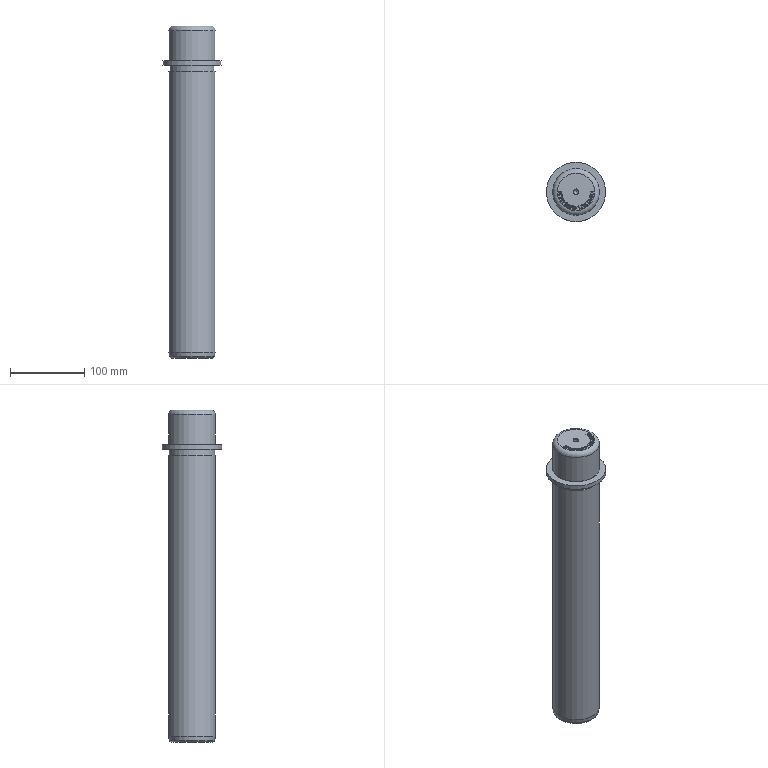Part | NX | features solid 2 | 1 solid | 313 faces | box 80 x 80 x 447 mm | volume 1398714 mm3 | spline 166 | plane 134 | cylinder 7 | cone 4 | torus 2 | commonest cylinder face diameters 6.647 x2 61 x2 63 x2 80 x1